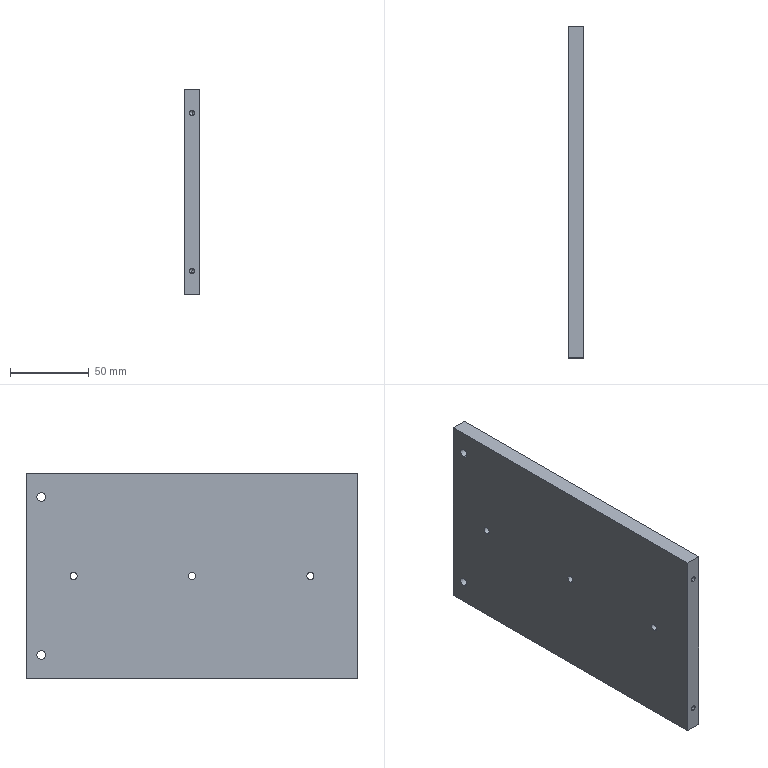Part | STEP file | 0243_205_Plate | 1 solid | 24 faces | box 10 x 210 x 130 mm | volume 271869 mm3 | cylinder 14 | plane 6 | cone 4 | commonest cylinder face diameters 4.5 x6 3.3 x4 5.5 x4